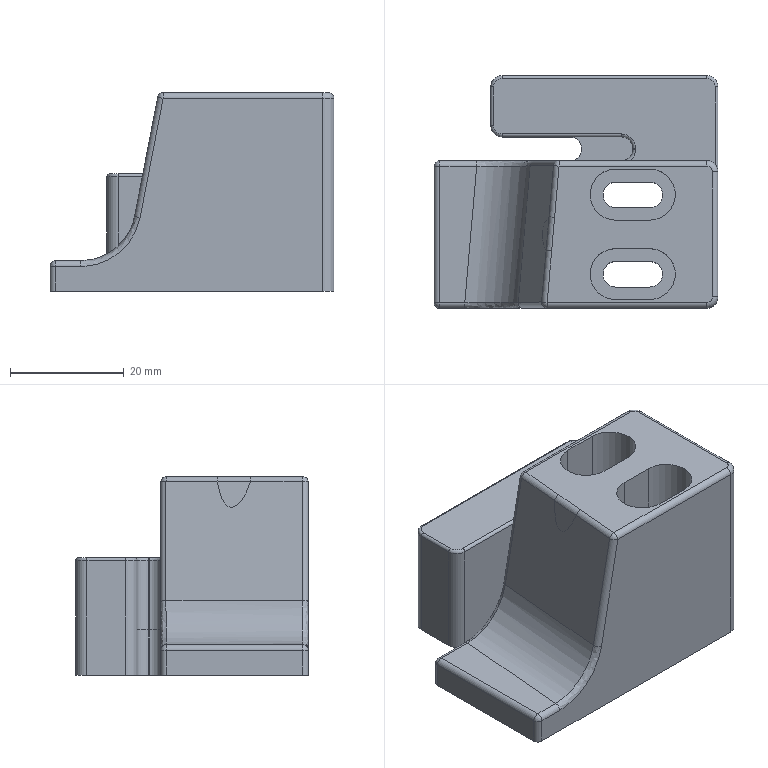NC program | NX | posted with a generic post | part box 50 x 41 x 35 mm
Lines 1813 to 2708 of 6591:
(ZLEVEL_PROFILE_COPY_COPY_1_COPY , TOOL : D6)
N3612 T06 M6
N3614 G54
N3616 G17 G0 G90 X6.382 Y0.77 S9500 M3
N3618 G43 Z30. H6
N3620 Z1.5
N3622 G94 G1 X6.249 Y0.717 Z1.493 F1000.
N3624 X5.88 Y0.389 Z1.467
N3626 X5.618 Y-0.132 Z1.436
N3628 X5.626 Y-0.897 Z1.396
N3630 X6.028 Y-1.549 Z1.356
N3632 X6.709 Y-1.9 Z1.316
N3634 X13.291 Z0.971
N3636 X13.963 Y-1.557 Z0.931
N3638 X14.367 Y-0.921 Z0.892
N3640 X14.391 Y-0.168 Z0.852
N3642 X14.143 Y0.359 Z0.822
N3644 X13.766 Y0.707 Z0.795
N3646 X13.291 Y0.9 Z0.768
N3648 X6.709 Z0.423
N3650 X6.249 Y0.717 Z0.397
N3652 X5.88 Y0.389 Z0.371
N3654 X5.618 Y-0.132 Z0.341
N3656 X5.626 Y-0.897 Z0.3
N3658 X6.028 Y-1.549 Z0.26
N3660 X6.709 Y-1.9 Z0.22
N3662 X13.291 Z-0.125
N3664 X13.963 Y-1.557 Z-0.164
N3666 X14.367 Y-0.921 Z-0.204
N3668 X14.391 Y-0.168 Z-0.243
N3670 X14.143 Y0.359 Z-0.274
N3672 X13.766 Y0.707 Z-0.301
N3674 X13.291 Y0.9 Z-0.328
N3676 X10. Z-0.5
N3678 X7. F2200.
N3680 G3 X5.6 Y-0.5 R1.4
N3682 X7. Y-1.9 R1.4
N3684 G1 X13.
N3686 G3 X14.4 Y-0.5 R1.4
N3688 X13. Y0.9 R1.4
N3690 G1 X10.
N3692 X7.3 Z-0.587
N3694 X7.001 Y0.881 Z-0.596
N3696 X6.575 Y0.805 Z-0.61
N3698 X6.428 Y0.754 Z-0.615
N3700 X6.233 Y0.638 Z-0.623
N3702 X6.137 Y0.578 Z-0.626
N3704 X5.96 Y0.401 Z-0.635
N3706 X5.826 Y0.21 Z-0.642
N3708 X5.765 Y0.112 Z-0.646
N3710 X5.734 Y0.039 Z-0.649
N3712 X5.682 Y-0.113 Z-0.654
N3714 X5.635 Y-0.355 Z-0.662
N3716 X5.622 Y-0.476 Z-0.666
N3718 X5.624 Y-0.549 Z-0.668
N3720 X5.641 Y-0.695 Z-0.673
N3722 X5.7 Y-0.939 Z-0.681
N3724 X5.768 Y-1.121 Z-0.688
N3726 X5.845 Y-1.243 Z-0.692
N3728 X6.005 Y-1.445 Z-0.701
N3730 X6.143 Y-1.583 Z-0.707
N3732 X6.258 Y-1.656 Z-0.712
N3734 X6.457 Y-1.764 Z-0.719
N3736 X6.641 Y-1.829 Z-0.725
N3738 X6.805 Y-1.86 Z-0.731
N3740 X7.101 Y-1.9 Z-0.74
N3742 X7.4 Z-0.75
N3744 X10.1 Z-0.837
N3746 X10.4 Z-0.846
N3748 X10.7 Z-0.856
N3750 X11. Z-0.865
N3752 X11.3 Z-0.875
N3754 X11.6 Z-0.885
N3756 X11.9 Z-0.894
N3758 X12.2 Z-0.904
N3760 X12.5 Z-0.913
N3762 X12.8 Z-0.923
N3764 X13.223 Y-1.856 Z-0.937
N3766 X13.387 Y-1.818 Z-0.942
N3768 X13.616 Y-1.733 Z-0.95
N3770 X13.78 Y-1.63 Z-0.957
N3772 X13.901 Y-1.54 Z-0.962
N3774 X14.129 Y-1.283 Z-0.973
N3776 X14.254 Y-1.073 Z-0.981
N3778 X14.348 Y-0.791 Z-0.99
N3780 X14.4 Y-0.5 Z-1.
N3782 G3 X13. Y0.9 R1.4
N3784 G1 X10.
N3786 X7.3 Z-1.087
N3788 X7.001 Y0.88 Z-1.096
N3790 X6.575 Y0.804 Z-1.11
N3792 X6.428 Y0.754 Z-1.115
N3794 X6.233 Y0.638 Z-1.123
N3796 X6.138 Y0.578 Z-1.126
N3798 X5.96 Y0.401 Z-1.135
N3800 X5.826 Y0.21 Z-1.142
N3802 X5.763 Y0.113 Z-1.146
N3804 X5.682 Y-0.113 Z-1.154
N3806 X5.635 Y-0.355 Z-1.162
N3808 X5.622 Y-0.476 Z-1.166
N3810 X5.624 Y-0.549 Z-1.168
N3812 X5.641 Y-0.695 Z-1.173
N3814 X5.7 Y-0.939 Z-1.181
N3816 X5.768 Y-1.121 Z-1.188
N3818 X5.845 Y-1.243 Z-1.192
N3820 X6.005 Y-1.445 Z-1.201
N3822 X6.143 Y-1.582 Z-1.207
N3824 X6.258 Y-1.656 Z-1.212
N3826 X6.457 Y-1.764 Z-1.219
N3828 X6.641 Y-1.829 Z-1.225
N3830 X6.805 Y-1.86 Z-1.231
N3832 X7.101 Y-1.9 Z-1.24
N3834 X7.4 Z-1.25
N3836 X10.1 Z-1.337
N3838 X10.4 Y-1.899 Z-1.346
N3840 X10.7 Y-1.9 Z-1.356
N3842 X11. Y-1.899 Z-1.365
N3844 X11.3 Y-1.9 Z-1.375
N3846 X11.6 Y-1.899 Z-1.385
N3848 X11.9 Y-1.9 Z-1.394
N3850 X12.2 Y-1.899 Z-1.404
N3852 X12.5 Y-1.9 Z-1.413
N3854 X12.8 Z-1.423
N3856 X13.223 Y-1.856 Z-1.437
N3858 X13.387 Y-1.818 Z-1.442
N3860 X13.717 Y-1.67 Z-1.454
N3862 X13.901 Y-1.54 Z-1.462
N3864 X14.121 Y-1.293 Z-1.472
N3866 X14.253 Y-1.073 Z-1.481
N3868 X14.348 Y-0.791 Z-1.49
N3870 X14.4 Y-0.5 Z-1.5
N3872 G3 X13. Y0.9 R1.4
N3874 G1 X10.
N3876 X7.3 Z-1.587
N3878 X7.001 Y0.88 Z-1.596
N3880 X6.575 Y0.804 Z-1.61
N3882 X6.428 Y0.754 Z-1.615
N3884 X6.233 Y0.638 Z-1.623
N3886 X6.138 Y0.578 Z-1.626
N3888 X5.961 Y0.401 Z-1.635
N3890 X5.826 Y0.21 Z-1.642
N3892 X5.763 Y0.113 Z-1.646
N3894 X5.682 Y-0.113 Z-1.654
N3896 X5.635 Y-0.355 Z-1.662
N3898 X5.622 Y-0.476 Z-1.666
N3900 X5.624 Y-0.549 Z-1.668
N3902 X5.641 Y-0.695 Z-1.673
N3904 X5.7 Y-0.938 Z-1.681
N3906 X5.768 Y-1.121 Z-1.688
N3908 X5.845 Y-1.243 Z-1.692
N3910 X6.005 Y-1.445 Z-1.701
N3912 X6.143 Y-1.582 Z-1.707
N3914 X6.258 Y-1.656 Z-1.712
N3916 X6.457 Y-1.764 Z-1.719
N3918 X6.64 Y-1.829 Z-1.725
N3920 X6.805 Y-1.859 Z-1.731
N3922 X7.101 Y-1.9 Z-1.74
N3924 X7.4 Z-1.75
N3926 X10.1 Z-1.837
N3928 X10.4 Y-1.899 Z-1.846
N3930 X10.7 Y-1.9 Z-1.856
N3932 X11. Y-1.899 Z-1.865
N3934 X11.3 Y-1.9 Z-1.875
N3936 X11.6 Y-1.899 Z-1.885
N3938 X11.9 Y-1.9 Z-1.894
N3940 X12.2 Y-1.899 Z-1.904
N3942 X12.5 Y-1.9 Z-1.913
N3944 X12.8 Z-1.923
N3946 X13.223 Y-1.856 Z-1.937
N3948 X13.386 Y-1.818 Z-1.942
N3950 X13.717 Y-1.67 Z-1.954
N3952 X13.901 Y-1.54 Z-1.962
N3954 X14.121 Y-1.293 Z-1.972
N3956 X14.253 Y-1.073 Z-1.981
N3958 X14.348 Y-0.791 Z-1.99
N3960 X14.4 Y-0.5 Z-2.
N3962 G3 X13. Y0.9 R1.4
N3964 G1 X10.
N3966 X7.3 Z-2.087
N3968 X7.001 Y0.88 Z-2.096
N3970 X6.575 Y0.804 Z-2.11
N3972 X6.428 Y0.754 Z-2.115
N3974 X6.233 Y0.638 Z-2.123
N3976 X6.138 Y0.578 Z-2.126
N3978 X5.961 Y0.401 Z-2.135
N3980 X5.826 Y0.21 Z-2.142
N3982 X5.763 Y0.113 Z-2.146
N3984 X5.682 Y-0.113 Z-2.154
N3986 X5.635 Y-0.355 Z-2.162
N3988 X5.622 Y-0.475 Z-2.166
N3990 X5.624 Y-0.549 Z-2.168
N3992 X5.641 Y-0.695 Z-2.173
N3994 X5.7 Y-0.938 Z-2.181
N3996 X5.768 Y-1.12 Z-2.188
N3998 X5.845 Y-1.243 Z-2.192
N4000 X6.005 Y-1.445 Z-2.201
N4002 X6.143 Y-1.582 Z-2.207
N4004 X6.258 Y-1.656 Z-2.212
N4006 X6.456 Y-1.764 Z-2.219
N4008 X6.64 Y-1.828 Z-2.225
N4010 X6.805 Y-1.859 Z-2.231
N4012 X7.101 Y-1.9 Z-2.24
N4014 X7.4 Z-2.25
N4016 X10.1 Z-2.337
N4018 X10.4 Y-1.899 Z-2.346
N4020 X10.7 Y-1.9 Z-2.356
N4022 X11. Y-1.899 Z-2.365
N4024 X11.3 Y-1.9 Z-2.375
N4026 X11.6 Y-1.899 Z-2.385
N4028 X11.9 Y-1.9 Z-2.394
N4030 X12.2 Y-1.899 Z-2.404
N4032 X12.5 Y-1.9 Z-2.413
N4034 X12.8 Z-2.423
N4036 X13.223 Y-1.856 Z-2.437
N4038 X13.386 Y-1.818 Z-2.442
N4040 X13.716 Y-1.67 Z-2.454
N4042 X13.901 Y-1.54 Z-2.462
N4044 X14.121 Y-1.293 Z-2.472
N4046 X14.253 Y-1.073 Z-2.481
N4048 X14.348 Y-0.791 Z-2.49
N4050 X14.4 Y-0.5 Z-2.5
N4052 G3 X13. Y0.9 R1.4
N4054 G1 X10.
N4056 X7.3 Z-2.587
N4058 X7.001 Y0.88 Z-2.596
N4060 X6.575 Y0.804 Z-2.61
N4062 X6.428 Y0.754 Z-2.615
N4064 X6.233 Y0.638 Z-2.623
N4066 X6.138 Y0.578 Z-2.626
N4068 X5.961 Y0.401 Z-2.635
N4070 X5.826 Y0.21 Z-2.642
N4072 X5.763 Y0.113 Z-2.646
N4074 X5.683 Y-0.113 Z-2.654
N4076 X5.635 Y-0.354 Z-2.662
N4078 X5.622 Y-0.475 Z-2.666
N4080 X5.625 Y-0.549 Z-2.668
N4082 X5.641 Y-0.695 Z-2.673
N4084 X5.7 Y-0.938 Z-2.681
N4086 X5.768 Y-1.12 Z-2.688
N4088 X5.845 Y-1.243 Z-2.692
N4090 X6.005 Y-1.444 Z-2.701
N4092 X6.143 Y-1.582 Z-2.707
N4094 X6.258 Y-1.655 Z-2.712
N4096 X6.456 Y-1.763 Z-2.719
N4098 X6.64 Y-1.828 Z-2.725
N4100 X6.805 Y-1.859 Z-2.731
N4102 X7.101 Y-1.9 Z-2.74
N4104 X7.4 Z-2.75
N4106 X10.1 Z-2.837
N4108 X10.4 Y-1.899 Z-2.846
N4110 X10.7 Y-1.9 Z-2.856
N4112 X11. Y-1.899 Z-2.865
N4114 X11.3 Y-1.9 Z-2.875
N4116 X11.6 Y-1.899 Z-2.885
N4118 X11.9 Y-1.9 Z-2.894
N4120 X12.2 Y-1.899 Z-2.904
N4122 X12.5 Y-1.9 Z-2.913
N4124 X12.8 Z-2.923
N4126 X13.223 Y-1.856 Z-2.937
N4128 X13.386 Y-1.818 Z-2.942
N4130 X13.716 Y-1.67 Z-2.954
N4132 X13.901 Y-1.54 Z-2.962
N4134 X14.121 Y-1.293 Z-2.972
N4136 X14.253 Y-1.073 Z-2.981
N4138 X14.348 Y-0.791 Z-2.99
N4140 X14.4 Y-0.5 Z-3.
N4142 G3 X13. Y0.9 R1.4
N4144 G1 X10.
N4146 X7.3 Z-3.087
N4148 X7.001 Y0.88 Z-3.096
N4150 X6.575 Y0.804 Z-3.11
N4152 X6.428 Y0.753 Z-3.115
N4154 X6.234 Y0.638 Z-3.123
N4156 X6.138 Y0.578 Z-3.126
N4158 X5.961 Y0.401 Z-3.135
N4160 X5.826 Y0.21 Z-3.142
N4162 X5.764 Y0.113 Z-3.146
N4164 X5.683 Y-0.113 Z-3.154
N4166 X5.635 Y-0.354 Z-3.162
N4168 X5.622 Y-0.475 Z-3.166
N4170 X5.625 Y-0.548 Z-3.168
N4172 X5.641 Y-0.695 Z-3.173
N4174 X5.7 Y-0.938 Z-3.181
N4176 X5.768 Y-1.12 Z-3.188
N4178 X5.845 Y-1.243 Z-3.192
N4180 X6.005 Y-1.444 Z-3.201
N4182 X6.143 Y-1.581 Z-3.207
N4184 X6.258 Y-1.655 Z-3.212
N4186 X6.456 Y-1.763 Z-3.219
N4188 X6.639 Y-1.828 Z-3.225
N4190 X6.805 Y-1.859 Z-3.231
N4192 X7.101 Y-1.9 Z-3.24
N4194 X7.4 Z-3.25
N4196 X10.1 Z-3.337
N4198 X10.4 Y-1.899 Z-3.346
N4200 X10.7 Y-1.9 Z-3.356
N4202 X11. Y-1.899 Z-3.365
N4204 X11.3 Y-1.9 Z-3.375
N4206 X11.6 Y-1.899 Z-3.385
N4208 X11.9 Y-1.9 Z-3.394
N4210 X12.2 Y-1.899 Z-3.404
N4212 X12.5 Y-1.9 Z-3.413
N4214 X12.8 Z-3.423
N4216 X13.223 Y-1.856 Z-3.437
N4218 X13.386 Y-1.818 Z-3.442
N4220 X13.716 Y-1.67 Z-3.454
N4222 X13.901 Y-1.54 Z-3.462
N4224 X14.121 Y-1.294 Z-3.472
N4226 X14.253 Y-1.072 Z-3.481
N4228 X14.348 Y-0.791 Z-3.49
N4230 X14.4 Y-0.5 Z-3.5
N4232 G3 X13. Y0.9 R1.4
N4234 G1 X10.
N4236 X7.3 Z-3.587
N4238 X7.001 Y0.88 Z-3.596
N4240 X6.575 Y0.804 Z-3.61
N4242 X6.428 Y0.753 Z-3.615
N4244 X6.234 Y0.638 Z-3.623
N4246 X6.138 Y0.578 Z-3.626
N4248 X5.961 Y0.401 Z-3.635
N4250 X5.827 Y0.21 Z-3.642
N4252 X5.764 Y0.113 Z-3.646
N4254 X5.683 Y-0.113 Z-3.654
N4256 X5.636 Y-0.354 Z-3.662
N4258 X5.622 Y-0.475 Z-3.666
N4260 X5.625 Y-0.548 Z-3.668
N4262 X5.641 Y-0.695 Z-3.673
N4264 X5.7 Y-0.937 Z-3.681
N4266 X5.768 Y-1.12 Z-3.688
N4268 X5.845 Y-1.243 Z-3.692
N4270 X6.005 Y-1.444 Z-3.701
N4272 X6.143 Y-1.581 Z-3.707
N4274 X6.258 Y-1.655 Z-3.712
N4276 X6.456 Y-1.763 Z-3.719
N4278 X6.639 Y-1.828 Z-3.725
N4280 X6.805 Y-1.859 Z-3.731
N4282 X7.101 Y-1.9 Z-3.74
N4284 X7.4 Z-3.75
N4286 X10.1 Z-3.837
N4288 X10.4 Y-1.899 Z-3.846
N4290 X10.7 Y-1.9 Z-3.856
N4292 X11. Y-1.899 Z-3.865
N4294 X11.3 Y-1.9 Z-3.875
N4296 X11.6 Y-1.899 Z-3.885
N4298 X11.9 Y-1.9 Z-3.894
N4300 X12.2 Y-1.899 Z-3.904
N4302 X12.5 Y-1.9 Z-3.913
N4304 X12.8 Z-3.923
N4306 X13.223 Y-1.856 Z-3.937
N4308 X13.386 Y-1.818 Z-3.942
N4310 X13.716 Y-1.67 Z-3.954
N4312 X13.9 Y-1.54 Z-3.962
N4314 X14.12 Y-1.294 Z-3.972
N4316 X14.253 Y-1.072 Z-3.981
N4318 X14.348 Y-0.791 Z-3.99
N4320 X14.4 Y-0.5 Z-4.
N4322 G3 X13. Y0.9 R1.4
N4324 G1 X10.
N4326 X7.3 Z-4.087
N4328 X7.001 Y0.88 Z-4.096
N4330 X6.575 Y0.804 Z-4.11
N4332 X6.428 Y0.753 Z-4.115
N4334 X6.234 Y0.638 Z-4.123
N4336 X6.139 Y0.578 Z-4.126
N4338 X5.961 Y0.401 Z-4.135
N4340 X5.825 Y0.208 Z-4.142
N4342 X5.761 Y0.109 Z-4.146
N4344 X5.683 Y-0.113 Z-4.154
N4346 X5.636 Y-0.355 Z-4.162
N4348 X5.622 Y-0.476 Z-4.166
N4350 X5.625 Y-0.549 Z-4.168
N4352 X5.641 Y-0.695 Z-4.173
N4354 X5.7 Y-0.938 Z-4.181
N4356 X5.768 Y-1.12 Z-4.188
N4358 X5.845 Y-1.243 Z-4.192
N4360 X6.005 Y-1.444 Z-4.201
N4362 X6.143 Y-1.581 Z-4.207
N4364 X6.258 Y-1.655 Z-4.212
N4366 X6.455 Y-1.763 Z-4.219
N4368 X6.639 Y-1.828 Z-4.225
N4370 X6.805 Y-1.859 Z-4.231
N4372 X7.101 Y-1.9 Z-4.24
N4374 X7.4 Z-4.25
N4376 X10.1 Z-4.337
N4378 X10.4 Y-1.899 Z-4.346
N4380 X10.7 Y-1.9 Z-4.356
N4382 X11. Y-1.899 Z-4.365
N4384 X11.3 Y-1.9 Z-4.375
N4386 X11.6 Y-1.899 Z-4.385
N4388 X11.9 Y-1.9 Z-4.394
N4390 X12.2 Y-1.899 Z-4.404
N4392 X12.5 Y-1.9 Z-4.413
N4394 X12.8 Z-4.423
N4396 X13.222 Y-1.856 Z-4.437
N4398 X13.386 Y-1.817 Z-4.442
N4400 X13.716 Y-1.67 Z-4.454
N4402 X13.9 Y-1.54 Z-4.462
N4404 X14.058 Y-1.384 Z-4.469
N4406 X14.122 Y-1.295 Z-4.472
N4408 X14.168 Y-1.222 Z-4.475
N4410 X14.253 Y-1.072 Z-4.481
N4412 X14.348 Y-0.791 Z-4.49
N4414 X14.4 Y-0.5 Z-4.5
N4416 G3 X13. Y0.9 R1.4
N4418 G1 X10.
N4420 X7.3 Z-4.587
N4422 X7.001 Y0.88 Z-4.596
N4424 X6.574 Y0.803 Z-4.61
N4426 X6.428 Y0.753 Z-4.615
N4428 X6.234 Y0.638 Z-4.623
N4430 X6.139 Y0.578 Z-4.626
N4432 X5.961 Y0.401 Z-4.635
N4434 X5.825 Y0.208 Z-4.642
N4436 X5.762 Y0.109 Z-4.646
N4438 X5.683 Y-0.113 Z-4.654
N4440 X5.636 Y-0.355 Z-4.662
N4442 X5.623 Y-0.476 Z-4.666
N4444 X5.625 Y-0.549 Z-4.668
N4446 X5.641 Y-0.695 Z-4.673
N4448 X5.7 Y-0.937 Z-4.681
N4450 X5.768 Y-1.12 Z-4.688
N4452 X5.845 Y-1.242 Z-4.692
N4454 X6.004 Y-1.444 Z-4.701
N4456 X6.143 Y-1.581 Z-4.707
N4458 X6.258 Y-1.655 Z-4.712
N4460 X6.455 Y-1.763 Z-4.719
N4462 X6.639 Y-1.827 Z-4.725
N4464 X6.805 Y-1.859 Z-4.731
N4466 X7.101 Y-1.9 Z-4.74
N4468 X7.4 Z-4.75
N4470 X10.1 Z-4.837
N4472 X10.4 Y-1.899 Z-4.846
N4474 X10.7 Y-1.9 Z-4.856
N4476 X11. Y-1.899 Z-4.865
N4478 X11.3 Y-1.9 Z-4.875
N4480 X11.6 Y-1.899 Z-4.885
N4482 X11.9 Y-1.9 Z-4.894
N4484 X12.2 Y-1.899 Z-4.904
N4486 X12.5 Y-1.9 Z-4.913
N4488 X12.8 Z-4.923
N4490 X13.222 Y-1.856 Z-4.937
N4492 X13.386 Y-1.817 Z-4.942
N4494 X13.716 Y-1.67 Z-4.954
N4496 X13.9 Y-1.54 Z-4.962
N4498 X14.058 Y-1.384 Z-4.969
N4500 X14.122 Y-1.295 Z-4.972
N4502 X14.168 Y-1.222 Z-4.975
N4504 X14.253 Y-1.072 Z-4.981
N4506 X14.348 Y-0.791 Z-4.99
N4508 X14.4 Y-0.5 Z-5.
N4510 G3 X13. Y0.9 R1.4
N4512 G1 X10.
N4514 X7.3 Z-5.087
N4516 X7.001 Y0.88 Z-5.096
N4518 X6.574 Y0.803 Z-5.11
N4520 X6.428 Y0.753 Z-5.115
N4522 X6.234 Y0.638 Z-5.123
N4524 X6.139 Y0.578 Z-5.126
N4526 X5.961 Y0.401 Z-5.135
N4528 X5.826 Y0.208 Z-5.142
N4530 X5.762 Y0.109 Z-5.146
N4532 X5.683 Y-0.113 Z-5.154
N4534 X5.636 Y-0.355 Z-5.162
N4536 X5.623 Y-0.476 Z-5.166
N4538 X5.625 Y-0.549 Z-5.168
N4540 X5.641 Y-0.695 Z-5.173
N4542 X5.7 Y-0.937 Z-5.181
N4544 X5.768 Y-1.119 Z-5.188
N4546 X5.845 Y-1.242 Z-5.192
N4548 X6.004 Y-1.443 Z-5.201
N4550 X6.143 Y-1.581 Z-5.207
N4552 X6.258 Y-1.655 Z-5.212
N4554 X6.455 Y-1.762 Z-5.219
N4556 X6.638 Y-1.827 Z-5.225
N4558 X6.805 Y-1.859 Z-5.231
N4560 X7.101 Y-1.9 Z-5.24
N4562 X7.4 Z-5.25
N4564 X10.1 Z-5.337
N4566 X10.4 Y-1.899 Z-5.346
N4568 X10.7 Y-1.9 Z-5.356
N4570 X11. Y-1.899 Z-5.365
N4572 X11.3 Y-1.9 Z-5.375
N4574 X11.6 Y-1.899 Z-5.385
N4576 X11.9 Y-1.9 Z-5.394
N4578 X12.2 Y-1.899 Z-5.404
N4580 X12.5 Y-1.9 Z-5.413
N4582 X12.8 Z-5.423
N4584 X13.222 Y-1.855 Z-5.437
N4586 X13.386 Y-1.817 Z-5.442
N4588 X13.715 Y-1.67 Z-5.454
N4590 X13.9 Y-1.54 Z-5.462
N4592 X14.058 Y-1.384 Z-5.469
N4594 X14.122 Y-1.295 Z-5.472
N4596 X14.167 Y-1.222 Z-5.475
N4598 X14.253 Y-1.072 Z-5.481
N4600 X14.348 Y-0.791 Z-5.49
N4602 X14.4 Y-0.5 Z-5.5
N4604 G3 X13. Y0.9 R1.4
N4606 G1 X10.
N4608 X7.3 Z-5.587
N4610 X7.001 Y0.88 Z-5.596
N4612 X6.573 Y0.805 Z-5.61
N4614 X6.428 Y0.753 Z-5.615
N4616 X6.229 Y0.637 Z-5.623
N4618 X6.134 Y0.574 Z-5.627
N4620 X5.961 Y0.401 Z-5.635
N4622 X5.827 Y0.21 Z-5.642
N4624 X5.763 Y0.112 Z-5.646
N4626 X5.683 Y-0.113 Z-5.654
N4628 X5.636 Y-0.354 Z-5.662
N4630 X5.623 Y-0.475 Z-5.666
N4632 X5.625 Y-0.548 Z-5.668
N4634 X5.641 Y-0.695 Z-5.673
N4636 X5.7 Y-0.937 Z-5.681
N4638 X5.769 Y-1.12 Z-5.688
N4640 X5.845 Y-1.242 Z-5.692
N4642 X6.004 Y-1.443 Z-5.701
N4644 X6.141 Y-1.582 Z-5.707
N4646 X6.258 Y-1.655 Z-5.712
N4648 X6.462 Y-1.765 Z-5.719
N4650 X6.645 Y-1.829 Z-5.725
N4652 X6.805 Y-1.859 Z-5.731
N4654 X7.101 Y-1.9 Z-5.74
N4656 X7.4 Z-5.75
N4658 X10.1 Z-5.837
N4660 X10.4 Y-1.899 Z-5.846
N4662 X10.7 Y-1.9 Z-5.856
N4664 X11. Y-1.899 Z-5.865
N4666 X11.3 Y-1.9 Z-5.875
N4668 X11.6 Y-1.899 Z-5.885
N4670 X11.9 Y-1.9 Z-5.894
N4672 X12.2 Y-1.899 Z-5.904
N4674 X12.5 Y-1.9 Z-5.913
N4676 X12.8 Z-5.923
N4678 X13.222 Y-1.855 Z-5.937
N4680 X13.386 Y-1.817 Z-5.942
N4682 X13.715 Y-1.67 Z-5.954
N4684 X13.9 Y-1.539 Z-5.962
N4686 X14.058 Y-1.384 Z-5.969
N4688 X14.122 Y-1.295 Z-5.972
N4690 X14.167 Y-1.222 Z-5.975
N4692 X14.253 Y-1.072 Z-5.981
N4694 X14.348 Y-0.791 Z-5.99
N4696 X14.4 Y-0.5 Z-6.
N4698 G3 X13. Y0.9 R1.4
N4700 G1 X10.
N4702 X7.3 Z-6.087
N4704 X7.001 Y0.88 Z-6.096
N4706 X6.573 Y0.805 Z-6.11
N4708 X6.428 Y0.753 Z-6.115
N4710 X6.229 Y0.637 Z-6.123
N4712 X6.134 Y0.574 Z-6.127
N4714 X5.961 Y0.401 Z-6.135
N4716 X5.827 Y0.21 Z-6.142
N4718 X5.764 Y0.112 Z-6.146
N4720 X5.683 Y-0.113 Z-6.154
N4722 X5.636 Y-0.354 Z-6.162
N4724 X5.623 Y-0.474 Z-6.166
N4726 X5.625 Y-0.548 Z-6.168
N4728 X5.641 Y-0.695 Z-6.173
N4730 X5.7 Y-0.937 Z-6.181
N4732 X5.769 Y-1.119 Z-6.188
N4734 X5.845 Y-1.242 Z-6.192
N4736 X6.003 Y-1.445 Z-6.201
N4738 X6.141 Y-1.582 Z-6.207
N4740 X6.258 Y-1.655 Z-6.212
N4742 X6.461 Y-1.764 Z-6.219
N4744 X6.645 Y-1.829 Z-6.225
N4746 X6.805 Y-1.859 Z-6.231
N4748 X7.101 Y-1.9 Z-6.24
N4750 X7.4 Z-6.25
N4752 X10.1 Z-6.337
N4754 X10.4 Y-1.899 Z-6.346
N4756 X10.7 Y-1.9 Z-6.356
N4758 X11. Y-1.899 Z-6.365
N4760 X11.3 Y-1.9 Z-6.375
N4762 X11.6 Y-1.899 Z-6.385
N4764 X11.9 Y-1.9 Z-6.394
N4766 X12.2 Y-1.899 Z-6.404
N4768 X12.5 Y-1.9 Z-6.413
N4770 X12.8 Z-6.423
N4772 X13.222 Y-1.855 Z-6.437
N4774 X13.386 Y-1.817 Z-6.442
N4776 X13.715 Y-1.67 Z-6.454
N4778 X13.9 Y-1.539 Z-6.462
N4780 X14.058 Y-1.384 Z-6.469
N4782 X14.121 Y-1.295 Z-6.472
N4784 X14.167 Y-1.222 Z-6.475
N4786 X14.253 Y-1.072 Z-6.481
N4788 X14.348 Y-0.791 Z-6.49
N4790 X14.4 Y-0.5 Z-6.5
N4792 G3 X13. Y0.9 R1.4
N4794 G1 X10.
N4796 X7.3 Z-6.587
N4798 X7.001 Y0.88 Z-6.596
N4800 X6.573 Y0.805 Z-6.61
N4802 X6.428 Y0.753 Z-6.615
N4804 X6.229 Y0.637 Z-6.623
N4806 X6.134 Y0.574 Z-6.627
N4808 X5.961 Y0.401 Z-6.635
N4810 X5.827 Y0.21 Z-6.642
N4812 X5.764 Y0.112 Z-6.646
N4814 X5.683 Y-0.113 Z-6.654
N4816 X5.636 Y-0.354 Z-6.662
N4818 X5.623 Y-0.474 Z-6.666
N4820 X5.625 Y-0.548 Z-6.668
N4822 X5.641 Y-0.695 Z-6.673
N4824 X5.7 Y-0.937 Z-6.681
N4826 X5.769 Y-1.119 Z-6.688
N4828 X5.845 Y-1.242 Z-6.692
N4830 X6.003 Y-1.445 Z-6.701
N4832 X6.141 Y-1.582 Z-6.707
N4834 X6.258 Y-1.655 Z-6.712
N4836 X6.461 Y-1.764 Z-6.719
N4838 X6.645 Y-1.829 Z-6.725
N4840 X6.805 Y-1.859 Z-6.731
N4842 X7.101 Y-1.9 Z-6.74
N4844 X7.4 Z-6.75
N4846 X10.1 Z-6.837
N4848 X10.4 Y-1.899 Z-6.846
N4850 X10.7 Y-1.9 Z-6.856
N4852 X11. Y-1.899 Z-6.865
N4854 X11.3 Y-1.9 Z-6.875
N4856 X11.6 Y-1.899 Z-6.885
N4858 X11.9 Y-1.9 Z-6.894
N4860 X12.2 Y-1.899 Z-6.904
N4862 X12.5 Y-1.9 Z-6.913
N4864 X12.8 Z-6.923
N4866 X13.222 Y-1.855 Z-6.937
N4868 X13.386 Y-1.817 Z-6.942
N4870 X13.715 Y-1.67 Z-6.954
N4872 X13.9 Y-1.539 Z-6.962
N4874 X14.057 Y-1.384 Z-6.969
N4876 X14.121 Y-1.295 Z-6.972
N4878 X14.167 Y-1.222 Z-6.975
N4880 X14.253 Y-1.072 Z-6.981
N4882 X14.347 Y-0.791 Z-6.99
N4884 X14.4 Y-0.5 Z-7.
N4886 G3 X13. Y0.9 R1.4
N4888 G1 X10.
N4890 X7.3 Z-7.087
N4892 X7.001 Y0.88 Z-7.096
N4894 X6.573 Y0.805 Z-7.11
N4896 X6.428 Y0.753 Z-7.115
N4898 X6.229 Y0.637 Z-7.123
N4900 X6.134 Y0.574 Z-7.127
N4902 X5.961 Y0.401 Z-7.135
N4904 X5.827 Y0.21 Z-7.142
N4906 X5.764 Y0.112 Z-7.146
N4908 X5.683 Y-0.113 Z-7.154
N4910 X5.636 Y-0.353 Z-7.162
N4912 X5.623 Y-0.474 Z-7.166
N4914 X5.625 Y-0.548 Z-7.168
N4916 X5.641 Y-0.695 Z-7.173
N4918 X5.7 Y-0.937 Z-7.181
N4920 X5.769 Y-1.119 Z-7.188
N4922 X5.845 Y-1.242 Z-7.192
N4924 X6.003 Y-1.444 Z-7.201
N4926 X6.141 Y-1.581 Z-7.207
N4928 X6.258 Y-1.655 Z-7.212
N4930 X6.461 Y-1.764 Z-7.219
N4932 X6.644 Y-1.829 Z-7.225
N4934 X6.805 Y-1.859 Z-7.231
N4936 X7.101 Y-1.9 Z-7.24
N4938 X7.4 Z-7.25
N4940 X10.1 Z-7.337
N4942 X10.4 Y-1.899 Z-7.346
N4944 X10.7 Y-1.9 Z-7.356
N4946 X11. Y-1.899 Z-7.365
N4948 X11.3 Y-1.9 Z-7.375
N4950 X11.6 Y-1.899 Z-7.385
N4952 X11.9 Y-1.9 Z-7.394
N4954 X12.2 Y-1.899 Z-7.404
N4956 X12.5 Y-1.9 Z-7.413
N4958 X12.8 Z-7.423
N4960 X13.222 Y-1.855 Z-7.437
N4962 X13.386 Y-1.817 Z-7.442
N4964 X13.715 Y-1.67 Z-7.454
N4966 X13.9 Y-1.539 Z-7.462
N4968 X14.057 Y-1.384 Z-7.469
N4970 X14.121 Y-1.296 Z-7.472
N4972 X14.167 Y-1.222 Z-7.475
N4974 X14.253 Y-1.072 Z-7.481
N4976 X14.347 Y-0.791 Z-7.49
N4978 X14.4 Y-0.5 Z-7.5
N4980 G3 X13. Y0.9 R1.4
N4982 G1 X10.
N4984 X7.3 Z-7.587
N4986 X7.001 Y0.88 Z-7.596
N4988 X6.573 Y0.805 Z-7.61
N4990 X6.428 Y0.753 Z-7.615
N4992 X6.23 Y0.637 Z-7.623
N4994 X6.134 Y0.574 Z-7.627
N4996 X5.961 Y0.401 Z-7.635
N4998 X5.827 Y0.21 Z-7.642
N5000 X5.764 Y0.112 Z-7.646
N5002 X5.683 Y-0.113 Z-7.654
N5004 X5.636 Y-0.353 Z-7.662
N5006 X5.623 Y-0.474 Z-7.666
N5008 X5.625 Y-0.548 Z-7.668
N5010 X5.641 Y-0.695 Z-7.673
N5012 X5.7 Y-0.936 Z-7.681
N5014 X5.769 Y-1.119 Z-7.688
N5016 X5.845 Y-1.242 Z-7.692
N5018 X6.003 Y-1.444 Z-7.701
N5020 X6.141 Y-1.581 Z-7.707
N5022 X6.258 Y-1.655 Z-7.712
N5024 X6.46 Y-1.764 Z-7.719
N5026 X6.644 Y-1.828 Z-7.725
N5028 X6.805 Y-1.859 Z-7.731
N5030 X7.101 Y-1.9 Z-7.74
N5032 X7.4 Z-7.75
N5034 X10.1 Z-7.837
N5036 X10.4 Y-1.899 Z-7.846
N5038 X10.7 Y-1.9 Z-7.856
N5040 X11. Y-1.899 Z-7.865
N5042 X11.3 Y-1.9 Z-7.875
N5044 X11.6 Y-1.899 Z-7.885
N5046 X11.9 Y-1.9 Z-7.894
N5048 X12.2 Y-1.899 Z-7.904
N5050 X12.5 Y-1.9 Z-7.913
N5052 X12.8 Z-7.923
N5054 X13.222 Y-1.855 Z-7.937
N5056 X13.386 Y-1.817 Z-7.942
N5058 X13.714 Y-1.67 Z-7.954
N5060 X13.9 Y-1.539 Z-7.962
N5062 X14.057 Y-1.384 Z-7.969
N5064 X14.121 Y-1.296 Z-7.972
N5066 X14.167 Y-1.223 Z-7.975
N5068 X14.253 Y-1.072 Z-7.981
N5070 X14.347 Y-0.791 Z-7.99
N5072 X14.4 Y-0.5 Z-8.
N5074 G3 X13. Y0.9 R1.4
N5076 G1 X10.
N5078 X7.3 Z-8.087
N5080 X7.001 Y0.88 Z-8.096
N5082 X6.573 Y0.805 Z-8.11
N5084 X6.428 Y0.753 Z-8.115
N5086 X6.23 Y0.637 Z-8.123
N5088 X6.134 Y0.574 Z-8.127
N5090 X5.961 Y0.401 Z-8.135
N5092 X5.827 Y0.21 Z-8.142
N5094 X5.764 Y0.112 Z-8.146
N5096 X5.683 Y-0.113 Z-8.154
N5098 X5.637 Y-0.353 Z-8.162
N5100 X5.624 Y-0.473 Z-8.166
N5102 X5.626 Y-0.547 Z-8.168
N5104 X5.641 Y-0.695 Z-8.173
N5106 X5.7 Y-0.936 Z-8.181
N5108 X5.769 Y-1.118 Z-8.188
N5110 X5.845 Y-1.242 Z-8.192
N5112 X6.002 Y-1.444 Z-8.201
N5114 X6.141 Y-1.581 Z-8.207
N5116 X6.258 Y-1.655 Z-8.212
N5118 X6.46 Y-1.764 Z-8.219
N5120 X6.644 Y-1.828 Z-8.225
N5122 X6.805 Y-1.859 Z-8.231
N5124 X7.101 Y-1.9 Z-8.24
N5126 X7.4 Z-8.25
N5128 X10.1 Z-8.337
N5130 X10.4 Y-1.899 Z-8.346
N5132 X10.7 Y-1.9 Z-8.356
N5134 X11. Y-1.899 Z-8.365
N5136 X11.3 Y-1.9 Z-8.375
N5138 X11.6 Y-1.899 Z-8.385
N5140 X11.9 Y-1.9 Z-8.394
N5142 X12.2 Y-1.899 Z-8.404
N5144 X12.5 Y-1.9 Z-8.413
N5146 X12.8 Z-8.423
N5148 X13.221 Y-1.855 Z-8.437
N5150 X13.386 Y-1.817 Z-8.442
N5152 X13.714 Y-1.67 Z-8.454
N5154 X13.9 Y-1.539 Z-8.462
N5156 X14.057 Y-1.384 Z-8.469
N5158 X14.121 Y-1.296 Z-8.472
N5160 X14.166 Y-1.223 Z-8.475
N5162 X14.253 Y-1.072 Z-8.481
N5164 X14.347 Y-0.791 Z-8.49
N5166 X14.4 Y-0.5 Z-8.5
N5168 G3 X13. Y0.9 R1.4
N5170 G1 X10.
N5172 X7.3 Z-8.587
N5174 X7.001 Y0.88 Z-8.596
N5176 X6.573 Y0.805 Z-8.61
N5178 X6.428 Y0.753 Z-8.615
N5180 X6.23 Y0.637 Z-8.623
N5182 X6.135 Y0.574 Z-8.627
N5184 X5.961 Y0.401 Z-8.635
N5186 X5.827 Y0.21 Z-8.642
N5188 X5.764 Y0.112 Z-8.646
N5190 X5.683 Y-0.113 Z-8.654
N5192 X5.637 Y-0.353 Z-8.662
N5194 X5.624 Y-0.473 Z-8.666
N5196 X5.626 Y-0.547 Z-8.668
N5198 X5.641 Y-0.695 Z-8.673
N5200 X5.7 Y-0.936 Z-8.681
N5202 X5.769 Y-1.118 Z-8.688
N5204 X5.845 Y-1.242 Z-8.692
N5206 X6.002 Y-1.444 Z-8.701
N5208 X6.141 Y-1.581 Z-8.707
N5210 X6.258 Y-1.655 Z-8.712
N5212 X6.46 Y-1.763 Z-8.719
N5214 X6.643 Y-1.828 Z-8.725
N5216 X6.805 Y-1.859 Z-8.731
N5218 X7.101 Y-1.9 Z-8.74
N5220 X7.4 Z-8.75
N5222 X10.1 Z-8.837
N5224 X10.4 Y-1.899 Z-8.846
N5226 X10.7 Y-1.9 Z-8.856
N5228 X11. Y-1.899 Z-8.865
N5230 X11.3 Y-1.9 Z-8.875
N5232 X11.6 Y-1.899 Z-8.885
N5234 X11.9 Y-1.9 Z-8.894
N5236 X12.2 Y-1.899 Z-8.904
N5238 X12.5 Y-1.9 Z-8.913
N5240 X12.8 Z-8.923
N5242 X13.221 Y-1.855 Z-8.937
N5244 X13.386 Y-1.817 Z-8.942
N5246 X13.714 Y-1.67 Z-8.954
N5248 X13.9 Y-1.539 Z-8.962
N5250 X14.057 Y-1.384 Z-8.969
N5252 X14.12 Y-1.296 Z-8.972
N5254 X14.166 Y-1.223 Z-8.975
N5256 X14.253 Y-1.072 Z-8.981
N5258 X14.347 Y-0.791 Z-8.99
N5260 X14.4 Y-0.5 Z-9.
N5262 G3 X13. Y0.9 R1.4
N5264 G1 X10.
N5266 X7.3 Z-9.087
N5268 X7.001 Y0.88 Z-9.096
N5270 X6.573 Y0.804 Z-9.11
N5272 X6.428 Y0.753 Z-9.115
N5274 X6.23 Y0.637 Z-9.123
N5276 X6.135 Y0.574 Z-9.127
N5278 X5.961 Y0.4 Z-9.135
N5280 X5.824 Y0.208 Z-9.142
N5282 X5.762 Y0.109 Z-9.146
N5284 X5.683 Y-0.113 Z-9.154
N5286 X5.637 Y-0.354 Z-9.162
N5288 X5.624 Y-0.474 Z-9.166
N5290 X5.626 Y-0.548 Z-9.168
N5292 X5.642 Y-0.695 Z-9.173
N5294 X5.7 Y-0.936 Z-9.181
N5296 X5.769 Y-1.118 Z-9.188
N5298 X5.845 Y-1.242 Z-9.192
N5300 X6.002 Y-1.443 Z-9.201
N5302 X6.141 Y-1.581 Z-9.207
N5304 X6.258 Y-1.655 Z-9.212
N5306 X6.46 Y-1.763 Z-9.219
N5308 X6.643 Y-1.828 Z-9.225
N5310 X6.805 Y-1.859 Z-9.231
N5312 X7.101 Y-1.9 Z-9.24
N5314 X7.4 Z-9.25
N5316 X10.1 Z-9.337
N5318 X10.4 Y-1.899 Z-9.346
N5320 X10.7 Y-1.9 Z-9.356
N5322 X11. Y-1.899 Z-9.365
N5324 X11.3 Y-1.9 Z-9.375
N5326 X11.6 Y-1.899 Z-9.385
N5328 X11.9 Y-1.9 Z-9.394
N5330 X12.2 Y-1.899 Z-9.404
N5332 X12.5 Y-1.9 Z-9.413
N5334 X12.8 Z-9.423
N5336 X13.221 Y-1.855 Z-9.437
N5338 X13.386 Y-1.817 Z-9.442
N5340 X13.714 Y-1.67 Z-9.454
N5342 X13.9 Y-1.539 Z-9.462
N5344 X14.057 Y-1.384 Z-9.469
N5346 X14.12 Y-1.296 Z-9.472
N5348 X14.166 Y-1.223 Z-9.475
N5350 X14.253 Y-1.072 Z-9.481
N5352 X14.347 Y-0.791 Z-9.49
N5354 X14.4 Y-0.5 Z-9.5
N5356 G3 X13. Y0.9 R1.4
N5358 G1 X10.
N5360 X7.3 Z-9.587
N5362 X7.001 Y0.88 Z-9.596
N5364 X6.573 Y0.804 Z-9.61
N5366 X6.428 Y0.753 Z-9.615
N5368 X6.23 Y0.637 Z-9.623
N5370 X6.135 Y0.574 Z-9.627
N5372 X5.961 Y0.4 Z-9.635
N5374 X5.824 Y0.208 Z-9.642
N5376 X5.763 Y0.109 Z-9.646
N5378 X5.683 Y-0.113 Z-9.654
N5380 X5.637 Y-0.354 Z-9.662
N5382 X5.624 Y-0.474 Z-9.666
N5384 X5.626 Y-0.548 Z-9.668
N5386 X5.642 Y-0.695 Z-9.673
N5388 X5.7 Y-0.936 Z-9.681
N5390 X5.769 Y-1.118 Z-9.688
N5392 X5.845 Y-1.242 Z-9.692
N5394 X6.002 Y-1.443 Z-9.701
N5396 X6.14 Y-1.58 Z-9.707